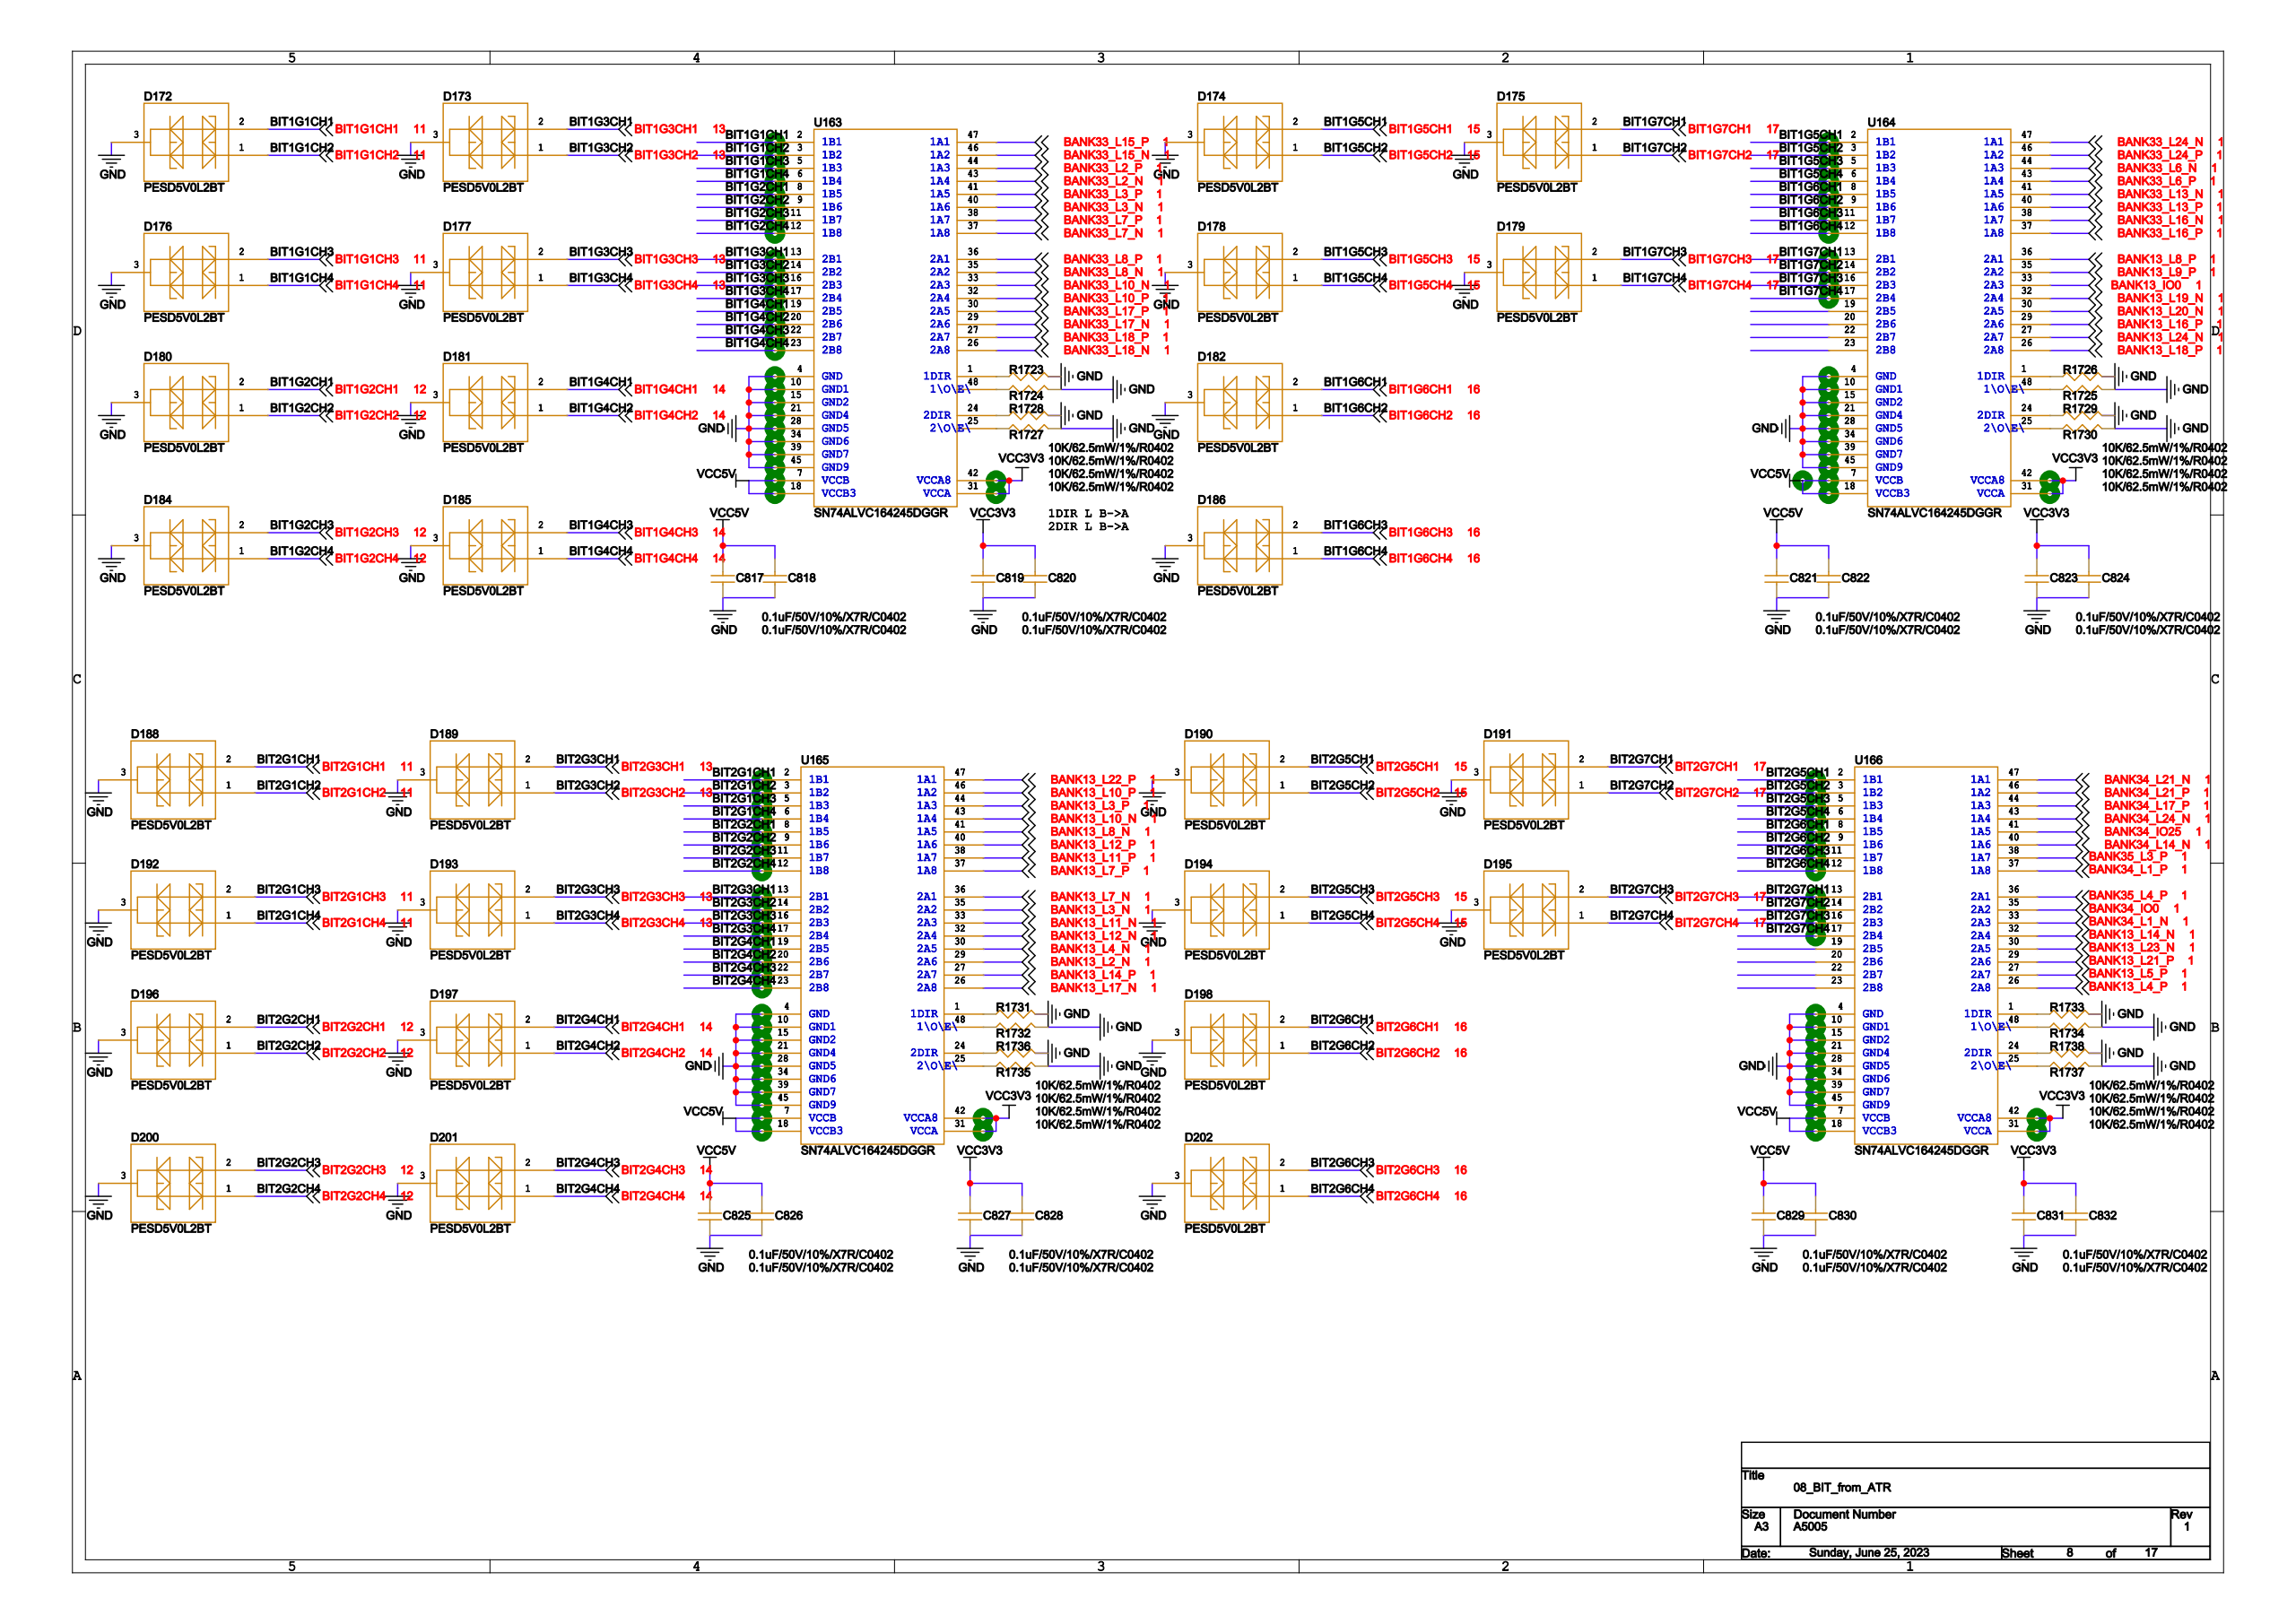Circuit board | Cadence Allegro | 2002 parts | 1538 nets | one sheet of the schematic
Parts on this sheet (reference | value | footprint):
C817 | 0.1uF/50V/10%/X7R/C0402 | 0402
C818 | 0.1uF/50V/10%/X7R/C0402 | 0402
C819 | 0.1uF/50V/10%/X7R/C0402 | 0402
C820 | 0.1uF/50V/10%/X7R/C0402 | 0402
C821 | 0.1uF/50V/10%/X7R/C0402 | 0402
C822 | 0.1uF/50V/10%/X7R/C0402 | 0402
C823 | 0.1uF/50V/10%/X7R/C0402 | 0402
C824 | 0.1uF/50V/10%/X7R/C0402 | 0402
C825 | 0.1uF/50V/10%/X7R/C0402 | 0402
C826 | 0.1uF/50V/10%/X7R/C0402 | 0402
C827 | 0.1uF/50V/10%/X7R/C0402 | 0402
C828 | 0.1uF/50V/10%/X7R/C0402 | 0402
C829 | 0.1uF/50V/10%/X7R/C0402 | 0402
C830 | 0.1uF/50V/10%/X7R/C0402 | 0402
C831 | 0.1uF/50V/10%/X7R/C0402 | 0402
C832 | 0.1uF/50V/10%/X7R/C0402 | 0402
D172 | PESD5V0L2BT | SOT23
D173 | PESD5V0L2BT | SOT23
D174 | PESD5V0L2BT | SOT23
D175 | PESD5V0L2BT | SOT23
D176 | PESD5V0L2BT | SOT23
D177 | PESD5V0L2BT | SOT23
D178 | PESD5V0L2BT | SOT23
D179 | PESD5V0L2BT | SOT23
D180 | PESD5V0L2BT | SOT23
D181 | PESD5V0L2BT | SOT23
D182 | PESD5V0L2BT | SOT23
D184 | PESD5V0L2BT | SOT23
D185 | PESD5V0L2BT | SOT23
D186 | PESD5V0L2BT | SOT23
D188 | PESD5V0L2BT | SOT23
D189 | PESD5V0L2BT | SOT23
D190 | PESD5V0L2BT | SOT23
D191 | PESD5V0L2BT | SOT23
D192 | PESD5V0L2BT | SOT23
D193 | PESD5V0L2BT | SOT23
D194 | PESD5V0L2BT | SOT23
D195 | PESD5V0L2BT | SOT23
D196 | PESD5V0L2BT | SOT23
D197 | PESD5V0L2BT | SOT23
D198 | PESD5V0L2BT | SOT23
D200 | PESD5V0L2BT | SOT23
D201 | PESD5V0L2BT | SOT23
D202 | PESD5V0L2BT | SOT23
R1723 | 10K/62.5mW/1%/R0402 | 0402
R1724 | 10K/62.5mW/1%/R0402 | 0402
R1725 | 10K/62.5mW/1%/R0402 | 0402
R1726 | 10K/62.5mW/1%/R0402 | 0402
R1727 | 10K/62.5mW/1%/R0402 | 0402
R1728 | 10K/62.5mW/1%/R0402 | 0402
R1729 | 10K/62.5mW/1%/R0402 | 0402
R1730 | 10K/62.5mW/1%/R0402 | 0402
R1731 | 10K/62.5mW/1%/R0402 | 0402
R1732 | 10K/62.5mW/1%/R0402 | 0402
R1733 | 10K/62.5mW/1%/R0402 | 0402
R1734 | 10K/62.5mW/1%/R0402 | 0402
R1735 | 10K/62.5mW/1%/R0402 | 0402
R1736 | 10K/62.5mW/1%/R0402 | 0402
R1737 | 10K/62.5mW/1%/R0402 | 0402
R1738 | 10K/62.5mW/1%/R0402 | 0402
U163 | SN74ALVC164245DGGR | TSSOP-48
U164 | SN74ALVC164245DGGR | TSSOP-48
U165 | SN74ALVC164245DGGR | TSSOP-48
U166 | SN74ALVC164245DGGR | TSSOP-48
Nets of these parts (net: part-pin ...):
3.3V: C819-2 C820-2 C823-2 C824-2 C827-2 C828-2 C831-2 C832-2 U163-31 U163-42 U164-31 U164-42 U165-31 U165-42 U166-31 U166-42
AGND: C817-1 C818-1 C819-1 C820-1 C821-1 C822-1 C823-1 C824-1 C825-1 C826-1 C827-1 C828-1 C829-1 C830-1 C831-1 C832-1 D172-3 D173-3 D174-3 D175-3 D176-3 D177-3 D178-3 D179-3 D180-3 D181-3 D182-3 D184-3 D185-3 D186-3 D188-3 D189-3 D190-3 D191-3 D192-3 D193-3 D194-3 D195-3 D196-3 D197-3 D198-3 D200-3 D201-3 D202-3 R1723-1 R1724-1 R1725-1 R1726-1 R1727-1 R1728-1 R1729-1 R1730-1 R1731-1 R1732-1 R1733-1 R1734-1 R1735-1 R1736-1 R1737-1 R1738-1 U163-4 U163-10 U163-15 U163-21 U163-28 U163-34 U163-39 U163-45 U164-4 U164-10 U164-15 U164-21 U164-28 U164-34 U164-39 U164-45 U165-4 U165-10 U165-15 U165-21 U165-28 U165-34 U165-39 U165-45 U166-4 U166-10 U166-15 U166-21 U166-28 U166-34 U166-39 U166-45
BANK33_L10_P: U163-32
BANK33_L17_P: U163-30
BANK33_L17_N: U163-29
BANK13_L4_P: U166-26
BANK33_L18_P: U163-27
BANK13_L5_P: U166-27
BANK33_L18_N: U163-26
BANK13_L21_P: U166-29
BANK13_L23_N: U166-30
BANK13_L14_N: U166-32
BANK34_L1_N: U166-33
BANK34_L21_P: U166-46
BANK34_L17_P: U166-44
BANK34_L24_N: U166-43
BANK34_IO25: U166-41
BANK34_L14_N: U166-40
BANK35_L3_P: U166-38
BANK34_L1_P: U166-37
BANK34_IO0: U166-35
BANK35_L4_P: U166-36
BANK34_L21_N: U166-47
BANK13_L22_P: U165-47
BANK13_L10_P: U165-46
BANK13_L3_P: U165-44
BANK13_L10_N: U165-43
BANK13_L8_N: U165-41
BANK13_L12_P: U165-40
BANK13_L11_P: U165-38
BANK13_L7_P: U165-37
BANK13_L7_N: U165-36
BANK13_L3_N: U165-35
BANK13_L11_N: U165-33
BANK13_L12_N: U165-32
BANK13_L4_N: U165-30
BANK13_L2_N: U165-29
BANK13_L14_P: U165-27
BANK13_L18_P: U164-26
BANK13_L17_N: U165-26
BANK13_L24_N: U164-27
BANK13_L16_P: U164-29
BANK13_L20_N: U164-30
BANK13_L19_N: U164-32
BANK13_IO0: U164-33
BANK13_L9_P: U164-35
BANK13_L8_P: U164-36
BANK33_L15_P: U163-47
BANK33_L16_P: U164-37
BANK33_L15_N: U163-46
BANK33_L16_N: U164-38
BANK33_L2_P: U163-44
BANK33_L13_P: U164-40
BANK33_L2_N: U163-43
BANK33_L13_N: U164-41
BANK33_L3_P: U163-41
BANK33_L6_P: U164-43
BANK33_L3_N: U163-40
BANK33_L6_N: U164-44
BANK33_L7_P: U163-38
BANK33_L24_P: U164-46
BANK33_L7_N: U163-37
BANK33_L24_N: U164-47
BANK33_L8_P: U163-36
BANK33_L8_N: U163-35
BANK33_L10_N: U163-33
VCC5V: C817-2 C818-2 C821-2 C822-2 C825-2 C826-2 C829-2 C830-2 U163-7 U163-18 U164-7 U164-18 U165-7 U165-18 U166-7 U166-18
BIT1G1CH1: D172-2 U163-2
BIT2G1CH1: D188-2 U165-2
BIT1G1CH2: D172-1 U163-3
BIT2G1CH2: D188-1 U165-3
BIT1G1CH4: D176-1 U163-6
BIT2G1CH4: D192-1 U165-6
BIT1G1CH3: D176-2 U163-5
BIT2G1CH3: D192-2 U165-5
BIT1G2CH2: D180-1 U163-9
BIT2G2CH2: D196-1 U165-9
BIT1G2CH4: D184-1 U163-12
BIT2G2CH4: D200-1 U165-12
BIT1G2CH3: D184-2 U163-11
BIT2G2CH3: D200-2 U165-11
BIT1G2CH1: D180-2 U163-8
BIT2G2CH1: D196-2 U165-8
BIT1G3CH2: D173-1 U163-14
BIT2G3CH2: D189-1 U165-14
BIT1G3CH4: D177-1 U163-17
BIT2G3CH4: D193-1 U165-17
BIT1G3CH3: D177-2 U163-16
BIT2G3CH3: D193-2 U165-16
BIT1G3CH1: D173-2 U163-13
BIT2G3CH1: D189-2 U165-13
BIT1G4CH2: D181-1 U163-20
BIT2G4CH2: D197-1 U165-20
BIT1G4CH4: D185-1 U163-23
BIT2G4CH4: D201-1 U165-23
BIT1G4CH3: D185-2 U163-22
BIT2G4CH3: D201-2 U165-22
BIT1G4CH1: D181-2 U163-19
BIT2G4CH1: D197-2 U165-19
BIT1G5CH2: D174-1 U164-3
BIT2G5CH2: D190-1 U166-3
BIT1G5CH4: D178-1 U164-6
BIT2G5CH4: D194-1 U166-6
BIT1G5CH3: D178-2 U164-5
BIT2G5CH3: D194-2 U166-5
BIT1G5CH1: D174-2 U164-2
BIT2G5CH1: D190-2 U166-2
BIT1G6CH2: D182-1 U164-9
BIT2G6CH2: D198-1 U166-9
BIT1G6CH4: D186-1 U164-12
BIT2G6CH4: D202-1 U166-12
BIT1G6CH3: D186-2 U164-11
BIT2G6CH3: D202-2 U166-11
BIT1G6CH1: D182-2 U164-8
BIT2G6CH1: D198-2 U166-8
BIT1G7CH2: D175-1 U164-14
BIT2G7CH2: D191-1 U166-14
BIT1G7CH4: D179-1 U164-17
BIT2G7CH4: D195-1 U166-17
BIT1G7CH3: D179-2 U164-16
BIT2G7CH3: D195-2 U166-16
BIT1G7CH1: D175-2 U164-13
BIT2G7CH1: D191-2 U166-13
N240386151: R1723-2 U163-1
N2403877347: R1724-2 U163-48
N2404532347: R1725-2 U164-48
N240451651: R1726-2 U164-1
N240386071: R1727-2 U163-25
N240385751: R1728-2 U163-24
N240451251: R1729-2 U164-24
N240451571: R1730-2 U164-25
N240482211: R1731-2 U165-1
N2404837947: R1732-2 U165-48
N240490171: R1733-2 U166-1
N2404917547: R1734-2 U166-48
N240482131: R1735-2 U165-25
N240481811: R1736-2 U165-24
N240490091: R1737-2 U166-25
N240489771: R1738-2 U166-24